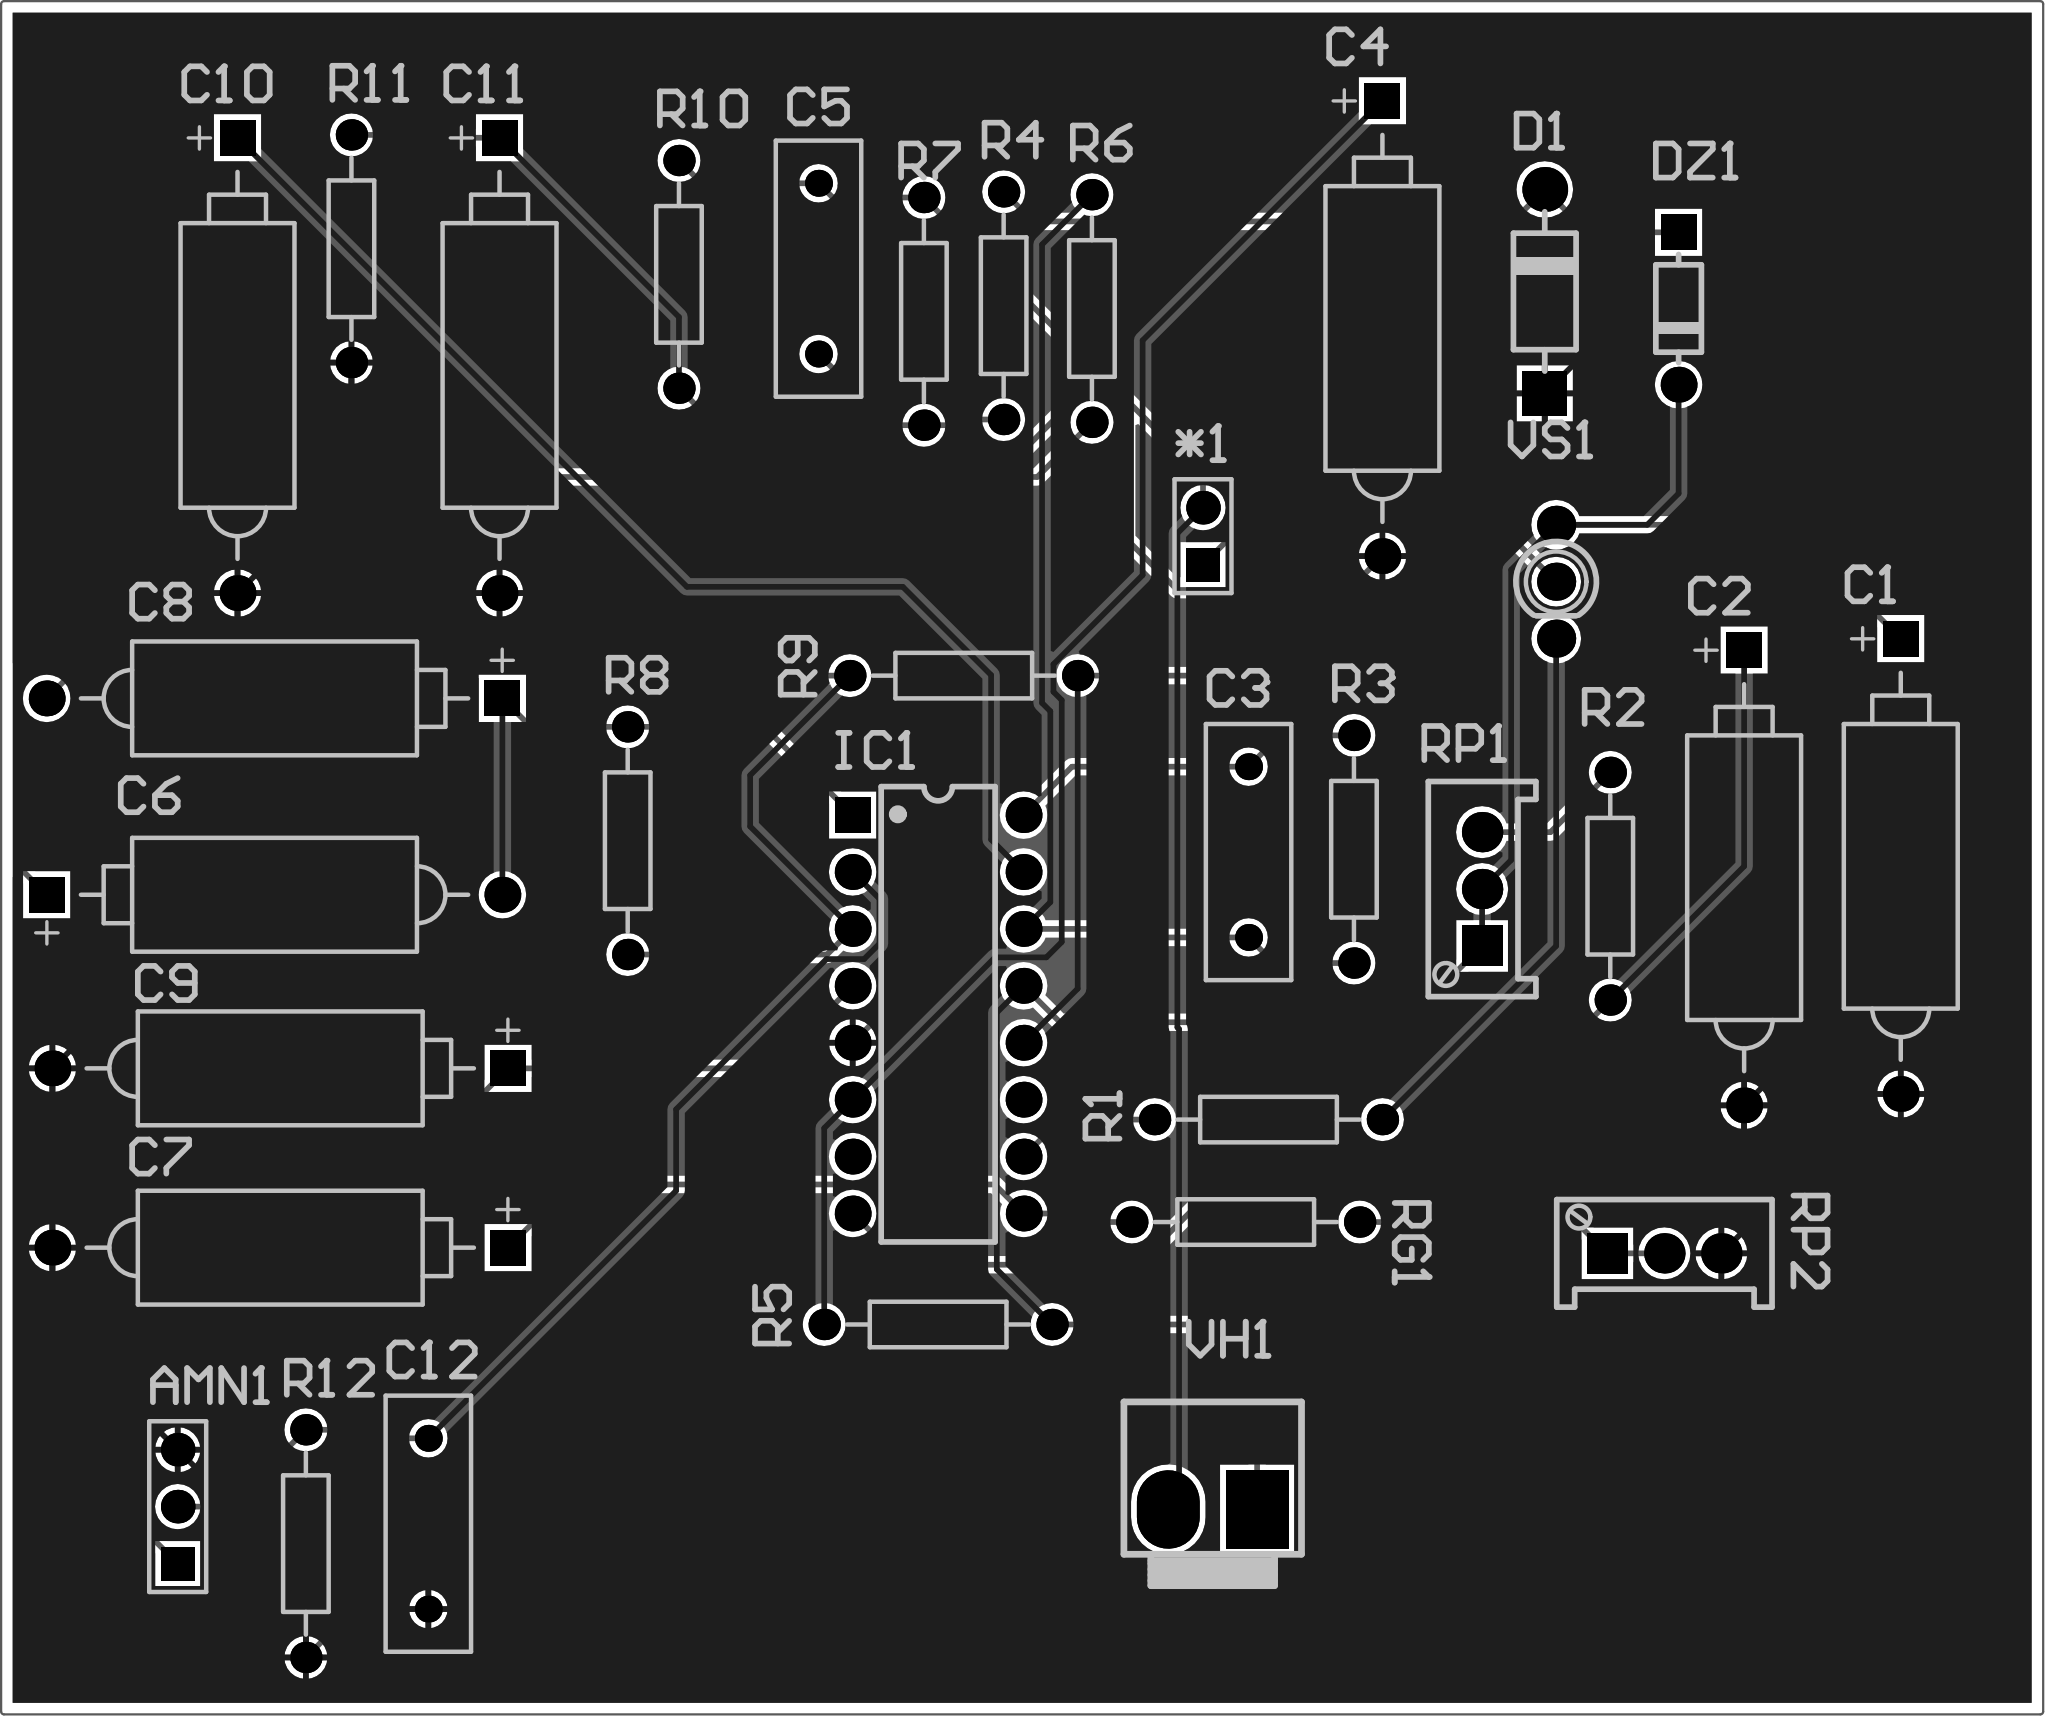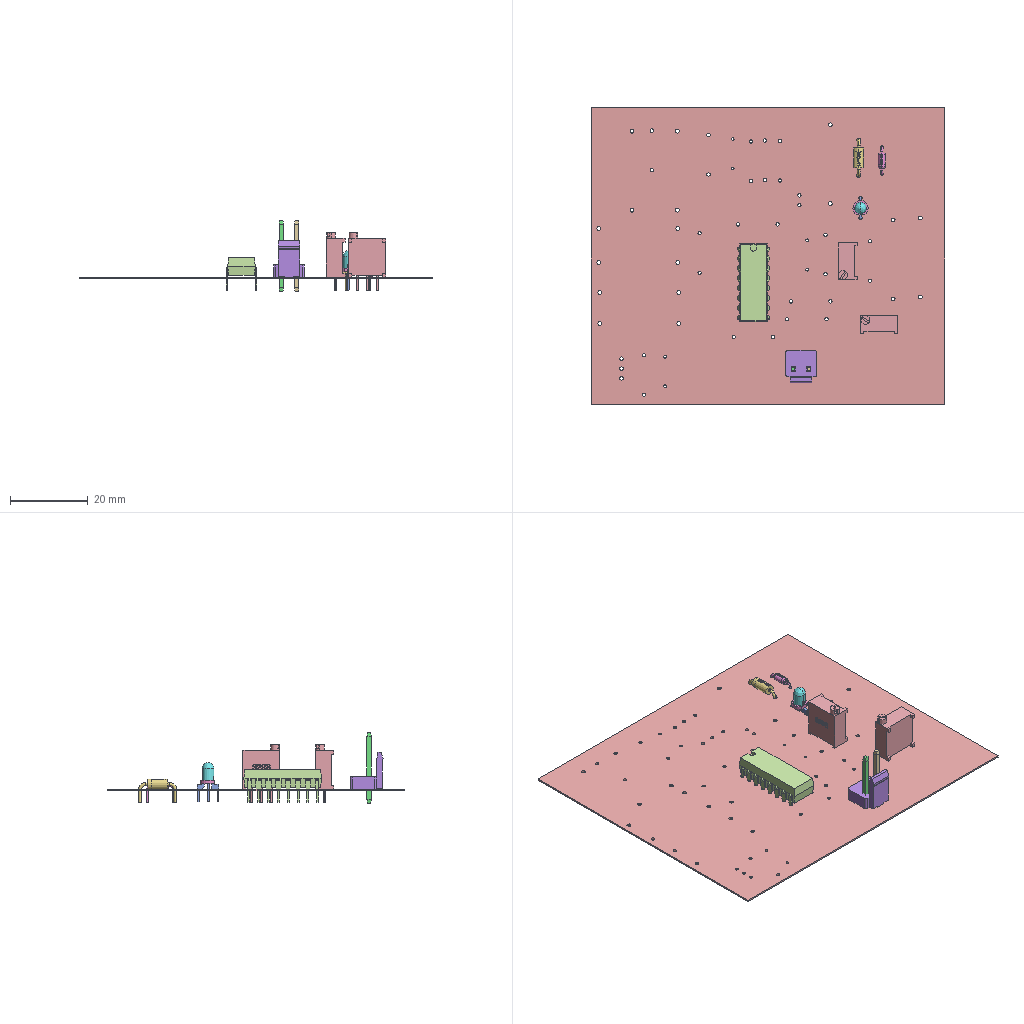Circuit board layout | Altium Designer | box 91.1 x 76.5 x 18.2 mm
Layer stack:
# Altium Designer layer stack of  (unit mm; dielectric type: 0 none, 1 core, 2 prepreg, 3 surface material)
index,name,kind,layer,copper_thickness_mm,dielectric_type,dielectric_thickness_mm,dielectric_material,dielectric_constant
0,Top Paste,other,,,,,,
1,Top Overlay,other,,,,,,
2,Top Solder,dielectric,,,3,0.0102,Solder Resist,3.5
3,Top Layer,copper,Top Layer,0.0356,,,,
4,Dielectric 1,dielectric,,,0,0.32,FR-4,4.8
5,Bottom Layer,copper,Bottom Layer,0.0356,,,,
6,Bottom Solder,dielectric,,,3,0.0102,Solder Resist,3.5
7,Bottom Overlay,other,,,,,,
8,Bottom Paste,other,,,,,,
# drill layer pairs: low layer,high layer
drill_pair,Top Layer,Bottom Layer
Part placement:
Designator,Comment,Layer,Footprint,Center-X(mm),Center-Y(mm),Rotation
VS1,1A/600V,TopLayer,LED_3mm-2P,127.381,79.375,270
VH1,220V,TopLayer,VH3.96-2A,112.066,37.973,180
RP2,1M,TopLayer,3296W,132.207,49.403,360
RP1,1M,TopLayer,3296W,124.079,65.659,90
RG1,10K,TopLayer,AXIAL-0.4,113.538,50.8,360
R12,47K,TopLayer,AXIAL-0.4,71.628,36.449,90
R11,470K,TopLayer,AXIAL-0.4,73.66,94.234,90
R10,1M,TopLayer,AXIAL-0.4,88.265,93.091,90
R9,15K,TopLayer,AXIAL-0.4,100.965,75.184,180
R8,320K,TopLayer,AXIAL-0.4,85.979,67.818,90
R7,100K,TopLayer,AXIAL-0.4,99.187,91.44,270
R6,15K,TopLayer,AXIAL-0.4,106.68,91.567,90
R5,100K,TopLayer,AXIAL-0.4,99.822,46.228,180
R4,47,TopLayer,AXIAL-0.4,102.743,91.694,90
R3,500K,TopLayer,AXIAL-0.4,118.364,67.437,90
R2,4.7K,TopLayer,AXIAL-0.4,129.794,65.786,270
R1,330K,TopLayer,AXIAL-0.4,114.554,55.372,180
IC1,TDH98072,TopLayer,DIP16,99.826,60.071,0
DZ1,5.1V,TopLayer,DO-35,132.842,91.567,270
D1,1N4007,TopLayer,DO-41,126.873,92.329,90
C12,0.01U,TopLayer,RAD-0.3,77.089,37.338,90
C11,33U,TopLayer,POLAR0.8,80.264,89.027,90
C10,22U,TopLayer,POLAR0.8,68.58,89.027,90
C9,100U,TopLayer,POLAR0.8,70.485,57.658,360
C8,1U,TopLayer,POLAR0.8,70.231,74.168,360
C7,4.7U,TopLayer,POLAR0.8,70.485,49.657,360
C6,47U,TopLayer,POLAR0.8,70.231,65.405,180
C5,0.1U,TopLayer,RAD-0.3,94.488,93.345,270
C4,4.7U,TopLayer,POLAR0.8,119.634,90.678,90
C3,0.047U,TopLayer,RAD-0.3,113.665,67.31,90
C2,100U,TopLayer,POLAR0.8,135.763,66.167,90
C1,470U,TopLayer,POLAR0.8,142.748,66.675,90
AMN1,PIR,TopLayer,HDR1X3,65.913,38.1,90
*1,H,TopLayer,HDR1X2,111.633,81.407,90
Pad and via stacks:
# Altium Designer via and pad stacks of  (unit mm). Each distinct definition once, with the count of objects using it.
# via: kind,start_layer,end_layer,hole_mm,diameter_mm,mode(0 simple;1 top-mid-bottom;2 full stack),diameter_per_layer,count,example_net
# pad: kind,layer,hole_mm,hole_type(0 round;1 square;2 slot),plating,top_size,top_shape(1 round;2 rect;3 octagon;9 rounded rect),mid_size,bottom_size,mode,footprint,size_per_layer,count,example
pad,Multi-Layer,1,0,plated,1.6x1.6,1,1.6x1.6,1.6x1.6,0,POLAR0.8,,9,C1.2
pad,Multi-Layer,1,0,plated,1.6x1.6,2,1.6x1.6,1.6x1.6,0,POLAR0.8,,9,C1.1
pad,Multi-Layer,0.8,0,plated,1.6x1.6,1,1.6x1.6,1.6x1.6,0,DO-35,,1,DZ1.2
pad,Multi-Layer,0.8,0,plated,1.6x1.6,2,1.6x1.6,1.6x1.6,0,DO-35,,1,DZ1.1
pad,Multi-Layer,1,0,plated,2x2,1,2x2,2x2,0,DO-41,,1,D1.2
pad,Multi-Layer,1,0,plated,2x2,2,2x2,2x2,0,DO-41,,1,D1.1
pad,Multi-Layer,0.8128,0,plated,1.6x1.6,2,1.6x1.6,1.6x1.6,0,DIP16,,1,IC1.1
pad,Multi-Layer,0.8128,0,plated,1.6x1.6,1,1.6x1.6,1.6x1.6,0,DIP16,,15,IC1.2
pad,Multi-Layer,0.85,0,plated,1.4x1.4,1,1.4x1.4,1.4x1.4,0,AXIAL-0.4,,26,R1.1
pad,Multi-Layer,1.6,0,plated,2.8x3.5,2,2.8x3.5,2.8x3.5,0,VH3.96-2A,,1,VH1.1
pad,Multi-Layer,1.6,0,plated,2.8x3.5,1,2.8x3.5,2.8x3.5,0,VH3.96-2A,,1,VH1.2
pad,Multi-Layer,0.9,0,plated,1.7x1.7,1,1.7x1.7,1.7x1.7,0,LED 3mm-2P,,3,VS1.2
pad,Multi-Layer,0.7,0,plated,1.8x1.8,1,1.8x1.8,1.8x1.8,0,3296W,,4,RP1.3
pad,Multi-Layer,0.7,0,plated,1.8x1.8,2,1.8x1.8,1.8x1.8,0,3296W,,2,RP1.1
pad,Multi-Layer,0.7,0,plated,1.2x1.2,1,1.2x1.2,1.2x1.2,0,RAD-0.3,,6,C3.2
pad,Multi-Layer,0.9,0,plated,1.5x1.5,2,1.5x1.5,1.5x1.5,0,HDR1X2,,1,*1.1
pad,Multi-Layer,0.9,0,plated,1.5x1.5,1,1.5x1.5,1.5x1.5,0,HDR1X2,,1,*1.2
pad,Multi-Layer,0.9,0,plated,1.5x1.5,2,1.5x1.5,1.5x1.5,0,HDR1X3,,1,AMN1.1
pad,Multi-Layer,0.9,0,plated,1.5x1.5,1,1.5x1.5,1.5x1.5,0,HDR1X3,,2,AMN1.2
Copper pours:
name,layer,net,type(0 solid;1 hatched;2 none)
D,Top Layer,GND,0
D,Bottom Layer,GND,0
Design rules, without the lines most boards share:
# Altium Designer design rules of  (exported by Altium Designer, unit mm)
# columns: name | kind | enabled | priority | scope1 | scope2 | descriptor | typed fields (field=value)
HoleToHoleClearance | 52 | enabled | 1 | All | All | Hole To Hole Clearance (Gap=10mil) (All),(All) | gap=0.254
DiffPairsRouting | 51 | enabled | 1 | All | All | Differential Pairs Uncoupled Length using the Gap Constraints (Min=10mil) (Max=10mil) (Prefered=10mil)  and Width Constraints (Min=15mil) (Max=15mil) (Prefered=15mil) (All) |
SolderMaskExpansion | 13 | enabled | 1 | All | All | Solder Mask Expansion (Expansion =4mil) (All) | expansion=0.1016
PasteMaskExpansion | 14 | enabled | 1 | All | All | Paste Mask Expansion (Expansion =0mil) (All) | expansion=0
RoutingVias | 11 | enabled | 1 | All | All | Routing Via (MinHoleWidth=28mil) (MaxHoleWidth=28mil) (PreferredHoleWidth=28mil) (MinWidth=50mil) (MaxWidth=50mil) (PreferedWidth=50mil) (All) | via_min_hole=0.7112 via_max_hole=0.7112 via_preferred_diameter=1.27 via_preferred_hole=0.7112
Width | 2 | enabled | 1 | All | All | Width Constraint (Min=10mil) (Max=10mil) (Preferred=10mil) (All) |
PolygonConnect | 20 | enabled | 1 | All | All | Polygon Connect Rule(Relief Connect )(Conductor Width=10mil) (Relief Angle=90 Angle) (Entries=4) (Air Gap Width=10mil) (All),(All) | connect_style(0=relief,1=direct,2=none)=0 relief_conductor_width=0.254 relief_entries=4
PlaneConnect | 6 | enabled | 1 | All | All | Power Plane Connect Rule(Relief Connect )(Expansion=20mil) (Conductor Width=10mil) (Air Gap=10mil) (Entries=4) (All) | relief_conductor_width=0.254 relief_entries=4 relief_expansion=0.508
Clearance | 0 | enabled | 1 | All | All | Clearance Constraint (Gap=10mil) (All),(All) | gap=0.254
Classes set for this board:
# Altium Designer classes of  (member kind: 0 net, 1 component, 2 from-to, 3 pad, 4 layer, 5 differential pair, 6 design channel, 7 polygon, 8 structure, 9 xSignal)
# columns: class name | member kind | superclass | members
Sheet1 | 1 | no | *1; AMN1; C1; C2; C3; C4; C5; C6; C7; C8; C9; C10; C11; C12; D1; DZ1; IC1; R1; R2; R3; R4; R5; R6; R7; R8; R9; R10; R11; R12; RG1; RP1; RP2; VH1; VS1;